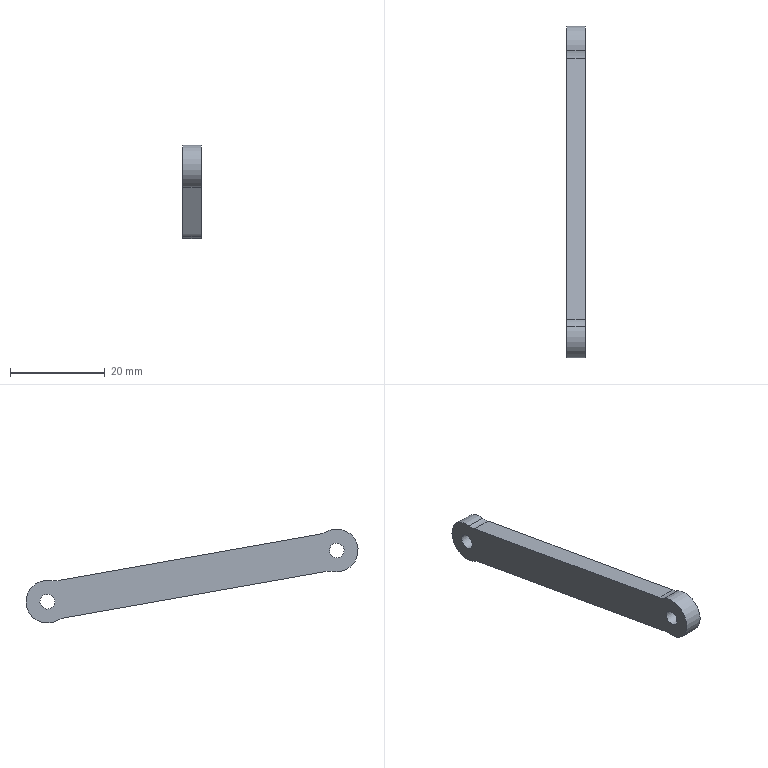Part | STEP file | Dodanie-wyci_gni_cie2_2 | 1 solid | 14 faces | box 4 x 70.047 x 19.826 mm | volume 2190 mm3 | cylinder 10 | plane 4 | commonest cylinder face diameters 9 x4 10 x4 3.1 x2
STEP:
#1=CARTESIAN_POINT('',(0.,0.,0.));
#2=DIRECTION('',(0.,0.,1.));
#3=DIRECTION('',(1.,0.,0.));
#4=AXIS2_PLACEMENT_3D('',#1,#2,#3);
#5=CARTESIAN_POINT('',(164.868,114.339,-98.824));
#6=VERTEX_POINT('',#5);
#7=CARTESIAN_POINT('',(164.868,114.609,-97.298));
#8=DIRECTION('',(1.,0.,0.));
#9=DIRECTION('',(0.,-0.1746,-0.9846));
#10=AXIS2_PLACEMENT_3D('',#7,#8,#9);
#11=CIRCLE('',#10,1.55);
#12=CARTESIAN_POINT('',(164.868,114.609,-97.298));
#13=DIRECTION('',(1.,0.,0.));
#14=DIRECTION('',(0.,-0.1746,-0.9846));
#15=AXIS2_PLACEMENT_3D('',#12,#13,#14);
#16=CYLINDRICAL_SURFACE('',#15,1.55);
#17=CARTESIAN_POINT('',(0.,0.));
#18=DIRECTION('',(1.,0.));
#19=VECTOR('',#18,1.);
#20=LINE('',#17,#19);
#21=(GEOMETRIC_REPRESENTATION_CONTEXT(2)PARAMETRIC_REPRESENTATION_CONTEXT()REPRESENTATION_CONTEXT('',''));
#22=DEFINITIONAL_REPRESENTATION('',(#20),#21);
#23=PCURVE('',#16,#22);
#24=CARTESIAN_POINT('',(164.868,145.133,-102.711));
#25=DIRECTION('',(1.,0.,0.));
#26=DIRECTION('',(0.,-0.1746,-0.9846));
#27=AXIS2_PLACEMENT_3D('',#24,#25,#26);
#28=PLANE('',#27);
#29=CARTESIAN_POINT('',(0.00000001,-31.));
#30=DIRECTION('',(1.,0.));
#31=AXIS2_PLACEMENT_2D('',#29,#30);
#32=CIRCLE('',#31,1.55);
#33=(GEOMETRIC_REPRESENTATION_CONTEXT(2)PARAMETRIC_REPRESENTATION_CONTEXT()REPRESENTATION_CONTEXT('',''));
#34=DEFINITIONAL_REPRESENTATION('',(#32),#33);
#35=PCURVE('',#28,#34);
#36=SURFACE_CURVE('',#11,(#23,#35),.PCURVE_S1.);
#37=EDGE_CURVE('',#6,#6,#36,.T.);
#38=ORIENTED_EDGE('',*,*,#37,.T.);
#39=CARTESIAN_POINT('',(168.868,114.339,-98.824));
#40=VERTEX_POINT('',#39);
#41=CARTESIAN_POINT('',(168.868,114.339,-98.824));
#42=DIRECTION('',(-1.,0.,0.));
#43=VECTOR('',#42,1.);
#44=LINE('',#41,#43);
#45=CARTESIAN_POINT('',(6.283,4.));
#46=DIRECTION('',(0.,-1.));
#47=VECTOR('',#46,1.);
#48=LINE('',#45,#47);
#49=(GEOMETRIC_REPRESENTATION_CONTEXT(2)PARAMETRIC_REPRESENTATION_CONTEXT()REPRESENTATION_CONTEXT('',''));
#50=DEFINITIONAL_REPRESENTATION('',(#48),#49);
#51=PCURVE('',#16,#50);
#52=CARTESIAN_POINT('',(0.,4.));
#53=DIRECTION('',(0.,-1.));
#54=VECTOR('',#53,1.);
#55=LINE('',#52,#54);
#56=(GEOMETRIC_REPRESENTATION_CONTEXT(2)PARAMETRIC_REPRESENTATION_CONTEXT()REPRESENTATION_CONTEXT('',''));
#57=DEFINITIONAL_REPRESENTATION('',(#55),#56);
#58=PCURVE('',#16,#57);
#59=SEAM_CURVE('',#44,(#51,#58),.PCURVE_S1.);
#60=EDGE_CURVE('',#40,#6,#59,.T.);
#61=ORIENTED_EDGE('',*,*,#60,.F.);
#62=CARTESIAN_POINT('',(168.868,114.609,-97.298));
#63=DIRECTION('',(-1.,0.,0.));
#64=DIRECTION('',(0.,-0.1746,-0.9846));
#65=AXIS2_PLACEMENT_3D('',#62,#63,#64);
#66=CIRCLE('',#65,1.55);
#67=CARTESIAN_POINT('',(6.283,4.));
#68=DIRECTION('',(-1.,0.));
#69=VECTOR('',#68,1.);
#70=LINE('',#67,#69);
#71=(GEOMETRIC_REPRESENTATION_CONTEXT(2)PARAMETRIC_REPRESENTATION_CONTEXT()REPRESENTATION_CONTEXT('',''));
#72=DEFINITIONAL_REPRESENTATION('',(#70),#71);
#73=PCURVE('',#16,#72);
#74=CARTESIAN_POINT('',(168.868,145.133,-102.711));
#75=DIRECTION('',(1.,0.,0.));
#76=DIRECTION('',(0.,-0.1746,-0.9846));
#77=AXIS2_PLACEMENT_3D('',#74,#75,#76);
#78=PLANE('',#77);
#79=CARTESIAN_POINT('',(1.55,-31.));
#80=CARTESIAN_POINT('',(1.55,-33.685));
#81=CARTESIAN_POINT('',(-0.775,-32.342));
#82=CARTESIAN_POINT('',(-3.1,-31.));
#83=CARTESIAN_POINT('',(-0.775,-29.658));
#84=CARTESIAN_POINT('',(1.55,-28.315));
#85=CARTESIAN_POINT('',(1.55,-31.));
#86=(BOUNDED_CURVE()B_SPLINE_CURVE(2,(#79,#80,#81,#82,#83,#84,#85),.UNSPECIFIED.,.T.,.F.)B_SPLINE_CURVE_WITH_KNOTS((1,2,2,2,2,1),(-2.094,0.,2.094,4.189,6.283,8.378),.UNSPECIFIED.)CURVE()GEOMETRIC_REPRESENTATION_ITEM()RATIONAL_B_SPLINE_CURVE((1.,0.5,1.,0.5,1.,0.5,1.))REPRESENTATION_ITEM(''));
#87=(GEOMETRIC_REPRESENTATION_CONTEXT(2)PARAMETRIC_REPRESENTATION_CONTEXT()REPRESENTATION_CONTEXT('',''));
#88=DEFINITIONAL_REPRESENTATION('',(#86),#87);
#89=PCURVE('',#78,#88);
#90=SURFACE_CURVE('',#66,(#73,#89),.PCURVE_S1.);
#91=EDGE_CURVE('',#40,#40,#90,.T.);
#92=ORIENTED_EDGE('',*,*,#91,.T.);
#93=ORIENTED_EDGE('',*,*,#60,.T.);
#94=EDGE_LOOP('',(#38,#61,#92,#93));
#95=FACE_BOUND('',#94,.F.);
#96=ADVANCED_FACE('',(#95),#16,.F.);
#97=CARTESIAN_POINT('',(164.868,175.386,-109.65));
#98=VERTEX_POINT('',#97);
#99=CARTESIAN_POINT('',(164.868,175.657,-108.124));
#100=DIRECTION('',(1.,0.,0.));
#101=DIRECTION('',(0.,-0.1746,-0.9846));
#102=AXIS2_PLACEMENT_3D('',#99,#100,#101);
#103=CIRCLE('',#102,1.55);
#104=CARTESIAN_POINT('',(164.868,175.657,-108.124));
#105=DIRECTION('',(1.,0.,0.));
#106=DIRECTION('',(0.,-0.1746,-0.9846));
#107=AXIS2_PLACEMENT_3D('',#104,#105,#106);
#108=CYLINDRICAL_SURFACE('',#107,1.55);
#109=CARTESIAN_POINT('',(0.,0.));
#110=DIRECTION('',(1.,0.));
#111=VECTOR('',#110,1.);
#112=LINE('',#109,#111);
#113=(GEOMETRIC_REPRESENTATION_CONTEXT(2)PARAMETRIC_REPRESENTATION_CONTEXT()REPRESENTATION_CONTEXT('',''));
#114=DEFINITIONAL_REPRESENTATION('',(#112),#113);
#115=PCURVE('',#108,#114);
#116=CARTESIAN_POINT('',(-0.00000001,31.));
#117=DIRECTION('',(1.,0.));
#118=AXIS2_PLACEMENT_2D('',#116,#117);
#119=CIRCLE('',#118,1.55);
#120=(GEOMETRIC_REPRESENTATION_CONTEXT(2)PARAMETRIC_REPRESENTATION_CONTEXT()REPRESENTATION_CONTEXT('',''));
#121=DEFINITIONAL_REPRESENTATION('',(#119),#120);
#122=PCURVE('',#28,#121);
#123=SURFACE_CURVE('',#103,(#115,#122),.PCURVE_S1.);
#124=EDGE_CURVE('',#98,#98,#123,.T.);
#125=ORIENTED_EDGE('',*,*,#124,.T.);
#126=CARTESIAN_POINT('',(168.868,175.386,-109.65));
#127=VERTEX_POINT('',#126);
#128=CARTESIAN_POINT('',(168.868,175.386,-109.65));
#129=DIRECTION('',(-1.,0.,0.));
#130=VECTOR('',#129,1.);
#131=LINE('',#128,#130);
#132=CARTESIAN_POINT('',(6.283,4.));
#133=DIRECTION('',(0.,-1.));
#134=VECTOR('',#133,1.);
#135=LINE('',#132,#134);
#136=(GEOMETRIC_REPRESENTATION_CONTEXT(2)PARAMETRIC_REPRESENTATION_CONTEXT()REPRESENTATION_CONTEXT('',''));
#137=DEFINITIONAL_REPRESENTATION('',(#135),#136);
#138=PCURVE('',#108,#137);
#139=CARTESIAN_POINT('',(0.,4.));
#140=DIRECTION('',(0.,-1.));
#141=VECTOR('',#140,1.);
#142=LINE('',#139,#141);
#143=(GEOMETRIC_REPRESENTATION_CONTEXT(2)PARAMETRIC_REPRESENTATION_CONTEXT()REPRESENTATION_CONTEXT('',''));
#144=DEFINITIONAL_REPRESENTATION('',(#142),#143);
#145=PCURVE('',#108,#144);
#146=SEAM_CURVE('',#131,(#138,#145),.PCURVE_S1.);
#147=EDGE_CURVE('',#127,#98,#146,.T.);
#148=ORIENTED_EDGE('',*,*,#147,.F.);
#149=CARTESIAN_POINT('',(168.868,175.657,-108.124));
#150=DIRECTION('',(-1.,0.,0.));
#151=DIRECTION('',(0.,-0.1746,-0.9846));
#152=AXIS2_PLACEMENT_3D('',#149,#150,#151);
#153=CIRCLE('',#152,1.55);
#154=CARTESIAN_POINT('',(6.283,4.));
#155=DIRECTION('',(-1.,0.));
#156=VECTOR('',#155,1.);
#157=LINE('',#154,#156);
#158=(GEOMETRIC_REPRESENTATION_CONTEXT(2)PARAMETRIC_REPRESENTATION_CONTEXT()REPRESENTATION_CONTEXT('',''));
#159=DEFINITIONAL_REPRESENTATION('',(#157),#158);
#160=PCURVE('',#108,#159);
#161=CARTESIAN_POINT('',(1.55,31.));
#162=CARTESIAN_POINT('',(1.55,28.315));
#163=CARTESIAN_POINT('',(-0.775,29.658));
#164=CARTESIAN_POINT('',(-3.1,31.));
#165=CARTESIAN_POINT('',(-0.775,32.342));
#166=CARTESIAN_POINT('',(1.55,33.685));
#167=CARTESIAN_POINT('',(1.55,31.));
#168=(BOUNDED_CURVE()B_SPLINE_CURVE(2,(#161,#162,#163,#164,#165,#166,#167),.UNSPECIFIED.,.T.,.F.)B_SPLINE_CURVE_WITH_KNOTS((1,2,2,2,2,1),(-2.094,0.,2.094,4.189,6.283,8.378),.UNSPECIFIED.)CURVE()GEOMETRIC_REPRESENTATION_ITEM()RATIONAL_B_SPLINE_CURVE((1.,0.5,1.,0.5,1.,0.5,1.))REPRESENTATION_ITEM(''));
#169=(GEOMETRIC_REPRESENTATION_CONTEXT(2)PARAMETRIC_REPRESENTATION_CONTEXT()REPRESENTATION_CONTEXT('',''));
#170=DEFINITIONAL_REPRESENTATION('',(#168),#169);
#171=PCURVE('',#78,#170);
#172=SURFACE_CURVE('',#153,(#160,#171),.PCURVE_S1.);
#173=EDGE_CURVE('',#127,#127,#172,.T.);
#174=ORIENTED_EDGE('',*,*,#173,.T.);
#175=ORIENTED_EDGE('',*,*,#147,.T.);
#176=EDGE_LOOP('',(#125,#148,#174,#175));
#177=FACE_BOUND('',#176,.F.);
#178=ADVANCED_FACE('',(#177),#108,.F.);
#179=CARTESIAN_POINT('',(168.868,174.871,-112.555));
#180=VERTEX_POINT('',#179);
#181=CARTESIAN_POINT('',(164.868,174.871,-112.555));
#182=VERTEX_POINT('',#181);
#183=CARTESIAN_POINT('',(168.868,174.871,-112.555));
#184=DIRECTION('',(-1.,0.,0.));
#185=VECTOR('',#184,1.);
#186=LINE('',#183,#185);
#187=CARTESIAN_POINT('',(164.868,175.657,-108.124));
#188=DIRECTION('',(1.,0.,0.));
#189=DIRECTION('',(0.,-0.1746,-0.9846));
#190=AXIS2_PLACEMENT_3D('',#187,#188,#189);
#191=CYLINDRICAL_SURFACE('',#190,4.5);
#192=CARTESIAN_POINT('',(0.,4.));
#193=DIRECTION('',(0.,-1.));
#194=VECTOR('',#193,1.);
#195=LINE('',#192,#194);
#196=(GEOMETRIC_REPRESENTATION_CONTEXT(2)PARAMETRIC_REPRESENTATION_CONTEXT()REPRESENTATION_CONTEXT('',''));
#197=DEFINITIONAL_REPRESENTATION('',(#195),#196);
#198=PCURVE('',#191,#197);
#199=CARTESIAN_POINT('',(164.868,175.657,-108.124));
#200=DIRECTION('',(1.,0.,0.));
#201=DIRECTION('',(0.,-0.1746,-0.9846));
#202=AXIS2_PLACEMENT_3D('',#199,#200,#201);
#203=CYLINDRICAL_SURFACE('',#202,4.5);
#204=CARTESIAN_POINT('',(6.283,4.));
#205=DIRECTION('',(0.,-1.));
#206=VECTOR('',#205,1.);
#207=LINE('',#204,#206);
#208=(GEOMETRIC_REPRESENTATION_CONTEXT(2)PARAMETRIC_REPRESENTATION_CONTEXT()REPRESENTATION_CONTEXT('',''));
#209=DEFINITIONAL_REPRESENTATION('',(#207),#208);
#210=PCURVE('',#203,#209);
#211=SURFACE_CURVE('',#186,(#198,#210),.PCURVE_S1.);
#212=EDGE_CURVE('',#180,#182,#211,.T.);
#213=ORIENTED_EDGE('',*,*,#212,.T.);
#214=CARTESIAN_POINT('',(164.868,174.983,-103.675));
#215=VERTEX_POINT('',#214);
#216=CARTESIAN_POINT('',(164.868,175.657,-108.124));
#217=DIRECTION('',(1.,0.,0.));
#218=DIRECTION('',(0.,-0.1746,-0.9846));
#219=AXIS2_PLACEMENT_3D('',#216,#217,#218);
#220=CIRCLE('',#219,4.5);
#221=CARTESIAN_POINT('',(0.,0.));
#222=DIRECTION('',(1.,0.));
#223=VECTOR('',#222,1.);
#224=LINE('',#221,#223);
#225=(GEOMETRIC_REPRESENTATION_CONTEXT(2)PARAMETRIC_REPRESENTATION_CONTEXT()REPRESENTATION_CONTEXT('',''));
#226=DEFINITIONAL_REPRESENTATION('',(#224),#225);
#227=PCURVE('',#191,#226);
#228=CARTESIAN_POINT('',(-0.00000001,31.));
#229=DIRECTION('',(1.,0.));
#230=AXIS2_PLACEMENT_2D('',#228,#229);
#231=CIRCLE('',#230,4.5);
#232=(GEOMETRIC_REPRESENTATION_CONTEXT(2)PARAMETRIC_REPRESENTATION_CONTEXT()REPRESENTATION_CONTEXT('',''));
#233=DEFINITIONAL_REPRESENTATION('',(#231),#232);
#234=PCURVE('',#28,#233);
#235=SURFACE_CURVE('',#220,(#227,#234),.PCURVE_S1.);
#236=EDGE_CURVE('',#182,#215,#235,.T.);
#237=ORIENTED_EDGE('',*,*,#236,.T.);
#238=CARTESIAN_POINT('',(168.868,174.983,-103.675));
#239=VERTEX_POINT('',#238);
#240=CARTESIAN_POINT('',(164.868,174.983,-103.675));
#241=DIRECTION('',(1.,0.,0.));
#242=VECTOR('',#241,1.);
#243=LINE('',#240,#242);
#244=CARTESIAN_POINT('',(3.467,0.));
#245=DIRECTION('',(0.,1.));
#246=VECTOR('',#245,1.);
#247=LINE('',#244,#246);
#248=(GEOMETRIC_REPRESENTATION_CONTEXT(2)PARAMETRIC_REPRESENTATION_CONTEXT()REPRESENTATION_CONTEXT('',''));
#249=DEFINITIONAL_REPRESENTATION('',(#247),#248);
#250=PCURVE('',#191,#249);
#251=CARTESIAN_POINT('',(164.868,174.234,-98.731));
#252=DIRECTION('',(1.,0.,0.));
#253=DIRECTION('',(0.,-0.1746,-0.9846));
#254=AXIS2_PLACEMENT_3D('',#251,#252,#253);
#255=CYLINDRICAL_SURFACE('',#254,5.);
#256=CARTESIAN_POINT('',(0.3259,0.));
#257=DIRECTION('',(0.,1.));
#258=VECTOR('',#257,1.);
#259=LINE('',#256,#258);
#260=(GEOMETRIC_REPRESENTATION_CONTEXT(2)PARAMETRIC_REPRESENTATION_CONTEXT()REPRESENTATION_CONTEXT('',''));
#261=DEFINITIONAL_REPRESENTATION('',(#259),#260);
#262=PCURVE('',#255,#261);
#263=SURFACE_CURVE('',#243,(#250,#262),.PCURVE_S1.);
#264=EDGE_CURVE('',#215,#239,#263,.T.);
#265=ORIENTED_EDGE('',*,*,#264,.T.);
#266=CARTESIAN_POINT('',(168.868,175.657,-108.124));
#267=DIRECTION('',(1.,0.,0.));
#268=DIRECTION('',(0.,-0.1746,-0.9846));
#269=AXIS2_PLACEMENT_3D('',#266,#267,#268);
#270=CIRCLE('',#269,4.5);
#271=CARTESIAN_POINT('',(0.,4.));
#272=DIRECTION('',(1.,0.));
#273=VECTOR('',#272,1.);
#274=LINE('',#271,#273);
#275=(GEOMETRIC_REPRESENTATION_CONTEXT(2)PARAMETRIC_REPRESENTATION_CONTEXT()REPRESENTATION_CONTEXT('',''));
#276=DEFINITIONAL_REPRESENTATION('',(#274),#275);
#277=PCURVE('',#191,#276);
#278=CARTESIAN_POINT('',(-0.00000001,31.));
#279=DIRECTION('',(1.,0.));
#280=AXIS2_PLACEMENT_2D('',#278,#279);
#281=CIRCLE('',#280,4.5);
#282=(GEOMETRIC_REPRESENTATION_CONTEXT(2)PARAMETRIC_REPRESENTATION_CONTEXT()REPRESENTATION_CONTEXT('',''));
#283=DEFINITIONAL_REPRESENTATION('',(#281),#282);
#284=PCURVE('',#78,#283);
#285=SURFACE_CURVE('',#270,(#277,#284),.PCURVE_S1.);
#286=EDGE_CURVE('',#180,#239,#285,.T.);
#287=ORIENTED_EDGE('',*,*,#286,.F.);
#288=EDGE_LOOP('',(#213,#237,#265,#287));
#289=FACE_BOUND('',#288,.T.);
#290=ADVANCED_FACE('',(#289),#191,.T.);
#291=CARTESIAN_POINT('',(168.868,113.823,-101.729));
#292=VERTEX_POINT('',#291);
#293=CARTESIAN_POINT('',(164.868,113.823,-101.729));
#294=VERTEX_POINT('',#293);
#295=CARTESIAN_POINT('',(168.868,113.823,-101.729));
#296=DIRECTION('',(-1.,0.,0.));
#297=VECTOR('',#296,1.);
#298=LINE('',#295,#297);
#299=CARTESIAN_POINT('',(164.868,114.609,-97.298));
#300=DIRECTION('',(1.,0.,0.));
#301=DIRECTION('',(0.,-0.1746,-0.9846));
#302=AXIS2_PLACEMENT_3D('',#299,#300,#301);
#303=CYLINDRICAL_SURFACE('',#302,4.5);
#304=CARTESIAN_POINT('',(0.,4.));
#305=DIRECTION('',(0.,-1.));
#306=VECTOR('',#305,1.);
#307=LINE('',#304,#306);
#308=(GEOMETRIC_REPRESENTATION_CONTEXT(2)PARAMETRIC_REPRESENTATION_CONTEXT()REPRESENTATION_CONTEXT('',''));
#309=DEFINITIONAL_REPRESENTATION('',(#307),#308);
#310=PCURVE('',#303,#309);
#311=CARTESIAN_POINT('',(164.868,114.609,-97.298));
#312=DIRECTION('',(1.,0.,0.));
#313=DIRECTION('',(0.,-0.1746,-0.9846));
#314=AXIS2_PLACEMENT_3D('',#311,#312,#313);
#315=CYLINDRICAL_SURFACE('',#314,4.5);
#316=CARTESIAN_POINT('',(6.283,4.));
#317=DIRECTION('',(0.,-1.));
#318=VECTOR('',#317,1.);
#319=LINE('',#316,#318);
#320=(GEOMETRIC_REPRESENTATION_CONTEXT(2)PARAMETRIC_REPRESENTATION_CONTEXT()REPRESENTATION_CONTEXT('',''));
#321=DEFINITIONAL_REPRESENTATION('',(#319),#320);
#322=PCURVE('',#315,#321);
#323=SURFACE_CURVE('',#298,(#310,#322),.PCURVE_S1.);
#324=EDGE_CURVE('',#292,#294,#323,.T.);
#325=ORIENTED_EDGE('',*,*,#324,.T.);
#326=CARTESIAN_POINT('',(164.868,115.283,-101.747));
#327=VERTEX_POINT('',#326);
#328=CARTESIAN_POINT('',(164.868,114.609,-97.298));
#329=DIRECTION('',(1.,0.,0.));
#330=DIRECTION('',(0.,-0.1746,-0.9846));
#331=AXIS2_PLACEMENT_3D('',#328,#329,#330);
#332=CIRCLE('',#331,4.5);
#333=CARTESIAN_POINT('',(0.,0.));
#334=DIRECTION('',(1.,0.));
#335=VECTOR('',#334,1.);
#336=LINE('',#333,#335);
#337=(GEOMETRIC_REPRESENTATION_CONTEXT(2)PARAMETRIC_REPRESENTATION_CONTEXT()REPRESENTATION_CONTEXT('',''));
#338=DEFINITIONAL_REPRESENTATION('',(#336),#337);
#339=PCURVE('',#303,#338);
#340=CARTESIAN_POINT('',(0.00000001,-31.));
#341=DIRECTION('',(1.,0.));
#342=AXIS2_PLACEMENT_2D('',#340,#341);
#343=CIRCLE('',#342,4.5);
#344=(GEOMETRIC_REPRESENTATION_CONTEXT(2)PARAMETRIC_REPRESENTATION_CONTEXT()REPRESENTATION_CONTEXT('',''));
#345=DEFINITIONAL_REPRESENTATION('',(#343),#344);
#346=PCURVE('',#28,#345);
#347=SURFACE_CURVE('',#332,(#339,#346),.PCURVE_S1.);
#348=EDGE_CURVE('',#294,#327,#347,.T.);
#349=ORIENTED_EDGE('',*,*,#348,.T.);
#350=CARTESIAN_POINT('',(168.868,115.283,-101.747));
#351=VERTEX_POINT('',#350);
#352=CARTESIAN_POINT('',(164.868,115.283,-101.747));
#353=DIRECTION('',(1.,0.,0.));
#354=VECTOR('',#353,1.);
#355=LINE('',#352,#354);
#356=CARTESIAN_POINT('',(0.3259,0.));
#357=DIRECTION('',(0.,1.));
#358=VECTOR('',#357,1.);
#359=LINE('',#356,#358);
#360=(GEOMETRIC_REPRESENTATION_CONTEXT(2)PARAMETRIC_REPRESENTATION_CONTEXT()REPRESENTATION_CONTEXT('',''));
#361=DEFINITIONAL_REPRESENTATION('',(#359),#360);
#362=PCURVE('',#303,#361);
#363=CARTESIAN_POINT('',(164.868,116.032,-106.691));
#364=DIRECTION('',(1.,0.,0.));
#365=DIRECTION('',(0.,-0.1746,-0.9846));
#366=AXIS2_PLACEMENT_3D('',#363,#364,#365);
#367=CYLINDRICAL_SURFACE('',#366,5.);
#368=CARTESIAN_POINT('',(3.467,0.));
#369=DIRECTION('',(0.,1.));
#370=VECTOR('',#369,1.);
#371=LINE('',#368,#370);
#372=(GEOMETRIC_REPRESENTATION_CONTEXT(2)PARAMETRIC_REPRESENTATION_CONTEXT()REPRESENTATION_CONTEXT('',''));
#373=DEFINITIONAL_REPRESENTATION('',(#371),#372);
#374=PCURVE('',#367,#373);
#375=SURFACE_CURVE('',#355,(#362,#374),.PCURVE_S1.);
#376=EDGE_CURVE('',#327,#351,#375,.T.);
#377=ORIENTED_EDGE('',*,*,#376,.T.);
#378=CARTESIAN_POINT('',(168.868,114.609,-97.298));
#379=DIRECTION('',(1.,0.,0.));
#380=DIRECTION('',(0.,-0.1746,-0.9846));
#381=AXIS2_PLACEMENT_3D('',#378,#379,#380);
#382=CIRCLE('',#381,4.5);
#383=CARTESIAN_POINT('',(0.,4.));
#384=DIRECTION('',(1.,0.));
#385=VECTOR('',#384,1.);
#386=LINE('',#383,#385);
#387=(GEOMETRIC_REPRESENTATION_CONTEXT(2)PARAMETRIC_REPRESENTATION_CONTEXT()REPRESENTATION_CONTEXT('',''));
#388=DEFINITIONAL_REPRESENTATION('',(#386),#387);
#389=PCURVE('',#303,#388);
#390=CARTESIAN_POINT('',(0.00000001,-31.));
#391=DIRECTION('',(1.,0.));
#392=AXIS2_PLACEMENT_2D('',#390,#391);
#393=CIRCLE('',#392,4.5);
#394=(GEOMETRIC_REPRESENTATION_CONTEXT(2)PARAMETRIC_REPRESENTATION_CONTEXT()REPRESENTATION_CONTEXT('',''));
#395=DEFINITIONAL_REPRESENTATION('',(#393),#394);
#396=PCURVE('',#78,#395);
#397=SURFACE_CURVE('',#382,(#389,#396),.PCURVE_S1.);
#398=EDGE_CURVE('',#292,#351,#397,.T.);
#399=ORIENTED_EDGE('',*,*,#398,.F.);
#400=EDGE_LOOP('',(#325,#349,#377,#399));
#401=FACE_BOUND('',#400,.T.);
#402=ADVANCED_FACE('',(#401),#303,.T.);
#403=ORIENTED_EDGE('',*,*,#91,.T.);
#404=EDGE_LOOP('',(#403));
#405=FACE_BOUND('',#404,.T.);
#406=ORIENTED_EDGE('',*,*,#173,.T.);
#407=EDGE_LOOP('',(#406));
#408=FACE_BOUND('',#407,.T.);
#409=CARTESIAN_POINT('',(168.868,173.361,-103.655));
#410=VERTEX_POINT('',#409);
#411=CARTESIAN_POINT('',(168.868,118.302,-93.89));
#412=VERTEX_POINT('',#411);
#413=CARTESIAN_POINT('',(168.868,173.361,-103.655));
#414=DIRECTION('',(0.,-0.9846,0.1746));
#415=VECTOR('',#414,1.);
#416=LINE('',#413,#415);
#417=CARTESIAN_POINT('',(-4.,27.959));
#418=DIRECTION('',(0.,-1.));
#419=VECTOR('',#418,1.);
#420=LINE('',#417,#419);
#421=(GEOMETRIC_REPRESENTATION_CONTEXT(2)PARAMETRIC_REPRESENTATION_CONTEXT()REPRESENTATION_CONTEXT('',''));
#422=DEFINITIONAL_REPRESENTATION('',(#420),#421);
#423=PCURVE('',#78,#422);
#424=CARTESIAN_POINT('',(166.868,145.831,-98.773));
#425=DIRECTION('',(0.,0.1746,0.9846));
#426=DIRECTION('',(1.,0.,0.));
#427=AXIS2_PLACEMENT_3D('',#424,#425,#426);
#428=PLANE('',#427);
#429=CARTESIAN_POINT('',(2.,27.959));
#430=DIRECTION('',(0.,-1.));
#431=VECTOR('',#430,1.);
#432=LINE('',#429,#431);
#433=(GEOMETRIC_REPRESENTATION_CONTEXT(2)PARAMETRIC_REPRESENTATION_CONTEXT()REPRESENTATION_CONTEXT('',''));
#434=DEFINITIONAL_REPRESENTATION('',(#432),#433);
#435=PCURVE('',#428,#434);
#436=SURFACE_CURVE('',#416,(#423,#435),.PCURVE_S1.);
#437=EDGE_CURVE('',#410,#412,#436,.T.);
#438=ORIENTED_EDGE('',*,*,#437,.T.);
#439=CARTESIAN_POINT('',(168.868,116.772,-93.352));
#440=VERTEX_POINT('',#439);
#441=CARTESIAN_POINT('',(168.868,119.175,-88.967));
#442=DIRECTION('',(-1.,0.,0.));
#443=DIRECTION('',(0.,-0.1746,-0.9846));
#444=AXIS2_PLACEMENT_3D('',#441,#442,#443);
#445=CIRCLE('',#444,5.);
#446=CARTESIAN_POINT('',(-4.,-27.959));
#447=CARTESIAN_POINT('',(-4.,-36.619));
#448=CARTESIAN_POINT('',(-11.5,-32.289));
#449=CARTESIAN_POINT('',(-19.,-27.959));
#450=CARTESIAN_POINT('',(-11.5,-23.628));
#451=CARTESIAN_POINT('',(-4.,-19.298));
#452=CARTESIAN_POINT('',(-4.,-27.959));
#453=(BOUNDED_CURVE()B_SPLINE_CURVE(2,(#446,#447,#448,#449,#450,#451,#452),.UNSPECIFIED.,.T.,.F.)B_SPLINE_CURVE_WITH_KNOTS((1,2,2,2,2,1),(-2.094,0.,2.094,4.189,6.283,8.378),.UNSPECIFIED.)CURVE()GEOMETRIC_REPRESENTATION_ITEM()RATIONAL_B_SPLINE_CURVE((1.,0.5,1.,0.5,1.,0.5,1.))REPRESENTATION_ITEM(''));
#454=(GEOMETRIC_REPRESENTATION_CONTEXT(2)PARAMETRIC_REPRESENTATION_CONTEXT()REPRESENTATION_CONTEXT('',''));
#455=DEFINITIONAL_REPRESENTATION('',(#453),#454);
#456=PCURVE('',#78,#455);
#457=CARTESIAN_POINT('',(164.868,119.175,-88.967));
#458=DIRECTION('',(1.,0.,0.));
#459=DIRECTION('',(0.,-0.1746,-0.9846));
#460=AXIS2_PLACEMENT_3D('',#457,#458,#459);
#461=CYLINDRICAL_SURFACE('',#460,5.);
#462=CARTESIAN_POINT('',(6.283,4.));
#463=DIRECTION('',(-1.,0.));
#464=VECTOR('',#463,1.);
#465=LINE('',#462,#464);
#466=(GEOMETRIC_REPRESENTATION_CONTEXT(2)PARAMETRIC_REPRESENTATION_CONTEXT()REPRESENTATION_CONTEXT('',''));
#467=DEFINITIONAL_REPRESENTATION('',(#465),#466);
#468=PCURVE('',#461,#467);
#469=SURFACE_CURVE('',#445,(#456,#468),.PCURVE_S1.);
#470=EDGE_CURVE('',#412,#440,#469,.T.);
#471=ORIENTED_EDGE('',*,*,#470,.T.);
#472=CARTESIAN_POINT('',(168.868,114.609,-97.298));
#473=DIRECTION('',(1.,0.,0.));
#474=DIRECTION('',(0.,-0.1746,-0.9846));
#475=AXIS2_PLACEMENT_3D('',#472,#473,#474);
#476=CIRCLE('',#475,4.5);
#477=CARTESIAN_POINT('',(0.00000001,-31.));
#478=DIRECTION('',(1.,0.));
#479=AXIS2_PLACEMENT_2D('',#477,#478);
#480=CIRCLE('',#479,4.5);
#481=(GEOMETRIC_REPRESENTATION_CONTEXT(2)PARAMETRIC_REPRESENTATION_CONTEXT()REPRESENTATION_CONTEXT('',''));
#482=DEFINITIONAL_REPRESENTATION('',(#480),#481);
#483=PCURVE('',#78,#482);
#484=CARTESIAN_POINT('',(0.,4.));
#485=DIRECTION('',(1.,0.));
#486=VECTOR('',#485,1.);
#487=LINE('',#484,#486);
#488=(GEOMETRIC_REPRESENTATION_CONTEXT(2)PARAMETRIC_REPRESENTATION_CONTEXT()REPRESENTATION_CONTEXT('',''));
#489=DEFINITIONAL_REPRESENTATION('',(#487),#488);
#490=PCURVE('',#315,#489);
#491=SURFACE_CURVE('',#476,(#483,#490),.PCURVE_S1.);
#492=EDGE_CURVE('',#440,#292,#491,.T.);
#493=ORIENTED_EDGE('',*,*,#492,.T.);
#494=ORIENTED_EDGE('',*,*,#398,.T.);
#495=CARTESIAN_POINT('',(168.868,116.905,-101.768));
#496=VERTEX_POINT('',#495);
#497=CARTESIAN_POINT('',(168.868,116.032,-106.691));
#498=DIRECTION('',(-1.,0.,0.));
#499=DIRECTION('',(0.,-0.1746,-0.9846));
#500=AXIS2_PLACEMENT_3D('',#497,#498,#499);
#501=CIRCLE('',#500,5.);
#502=CARTESIAN_POINT('',(14.,-27.959));
#503=CARTESIAN_POINT('',(14.,-36.619));
#504=CARTESIAN_POINT('',(6.5,-32.289));
#505=CARTESIAN_POINT('',(-1.,-27.959));
#506=CARTESIAN_POINT('',(6.5,-23.628));
#507=CARTESIAN_POINT('',(14.,-19.298));
#508=CARTESIAN_POINT('',(14.,-27.959));
#509=(BOUNDED_CURVE()B_SPLINE_CURVE(2,(#502,#503,#504,#505,#506,#507,#508),.UNSPECIFIED.,.T.,.F.)B_SPLINE_CURVE_WITH_KNOTS((1,2,2,2,2,1),(-2.094,0.,2.094,4.189,6.283,8.378),.UNSPECIFIED.)CURVE()GEOMETRIC_REPRESENTATION_ITEM()RATIONAL_B_SPLINE_CURVE((1.,0.5,1.,0.5,1.,0.5,1.))REPRESENTATION_ITEM(''));
#510=(GEOMETRIC_REPRESENTATION_CONTEXT(2)PARAMETRIC_REPRESENTATION_CONTEXT()REPRESENTATION_CONTEXT('',''));
#511=DEFINITIONAL_REPRESENTATION('',(#509),#510);
#512=PCURVE('',#78,#511);
#513=CARTESIAN_POINT('',(6.283,4.));
#514=DIRECTION('',(-1.,0.));
#515=VECTOR('',#514,1.);
#516=LINE('',#513,#515);
#517=(GEOMETRIC_REPRESENTATION_CONTEXT(2)PARAMETRIC_REPRESENTATION_CONTEXT()REPRESENTATION_CONTEXT('',''));
#518=DEFINITIONAL_REPRESENTATION('',(#516),#517);
#519=PCURVE('',#367,#518);
#520=SURFACE_CURVE('',#501,(#512,#519),.PCURVE_S1.);
#521=EDGE_CURVE('',#351,#496,#520,.T.);
#522=ORIENTED_EDGE('',*,*,#521,.T.);
#523=CARTESIAN_POINT('',(168.868,171.964,-111.532));
#524=VERTEX_POINT('',#523);
#525=CARTESIAN_POINT('',(168.868,116.905,-101.768));
#526=DIRECTION('',(0.,0.9846,-0.1746));
#527=VECTOR('',#526,1.);
#528=LINE('',#525,#527);
#529=CARTESIAN_POINT('',(4.,-27.959));
#530=DIRECTION('',(0.,1.));
#531=VECTOR('',#530,1.);
#532=LINE('',#529,#531);
#533=(GEOMETRIC_REPRESENTATION_CONTEXT(2)PARAMETRIC_REPRESENTATION_CONTEXT()REPRESENTATION_CONTEXT('',''));
#534=DEFINITIONAL_REPRESENTATION('',(#532),#533);
#535=PCURVE('',#78,#534);
#536=CARTESIAN_POINT('',(166.868,144.435,-106.65));
#537=DIRECTION('',(0.,-0.1746,-0.9846));
#538=DIRECTION('',(-1.,0.,0.));
#539=AXIS2_PLACEMENT_3D('',#536,#537,#538);
#540=PLANE('',#539);
#541=CARTESIAN_POINT('',(-2.,-27.959));
#542=DIRECTION('',(0.,1.));
#543=VECTOR('',#542,1.);
#544=LINE('',#541,#543);
#545=(GEOMETRIC_REPRESENTATION_CONTEXT(2)PARAMETRIC_REPRESENTATION_CONTEXT()REPRESENTATION_CONTEXT('',''));
#546=DEFINITIONAL_REPRESENTATION('',(#544),#545);
#547=PCURVE('',#540,#546);
#548=SURFACE_CURVE('',#528,(#535,#547),.PCURVE_S1.);
#549=EDGE_CURVE('',#496,#524,#548,.T.);
#550=ORIENTED_EDGE('',*,*,#549,.T.);
#551=CARTESIAN_POINT('',(168.868,173.494,-112.07));
#552=VERTEX_POINT('',#551);
#553=CARTESIAN_POINT('',(168.868,171.091,-116.455));
#554=DIRECTION('',(-1.,0.,0.));
#555=DIRECTION('',(0.,-0.1746,-0.9846));
#556=AXIS2_PLACEMENT_3D('',#553,#554,#555);
#557=CIRCLE('',#556,5.);
#558=CARTESIAN_POINT('',(14.,27.959));
#559=CARTESIAN_POINT('',(14.,19.298));
#560=CARTESIAN_POINT('',(6.5,23.628));
#561=CARTESIAN_POINT('',(-1.,27.959));
#562=CARTESIAN_POINT('',(6.5,32.289));
#563=CARTESIAN_POINT('',(14.,36.619));
#564=CARTESIAN_POINT('',(14.,27.959));
#565=(BOUNDED_CURVE()B_SPLINE_CURVE(2,(#558,#559,#560,#561,#562,#563,#564),.UNSPECIFIED.,.T.,.F.)B_SPLINE_CURVE_WITH_KNOTS((1,2,2,2,2,1),(-2.094,0.,2.094,4.189,6.283,8.378),.UNSPECIFIED.)CURVE()GEOMETRIC_REPRESENTATION_ITEM()RATIONAL_B_SPLINE_CURVE((1.,0.5,1.,0.5,1.,0.5,1.))REPRESENTATION_ITEM(''));
#566=(GEOMETRIC_REPRESENTATION_CONTEXT(2)PARAMETRIC_REPRESENTATION_CONTEXT()REPRESENTATION_CONTEXT('',''));
#567=DEFINITIONAL_REPRESENTATION('',(#565),#566);
#568=PCURVE('',#78,#567);
#569=CARTESIAN_POINT('',(164.868,171.091,-116.455));
#570=DIRECTION('',(1.,0.,0.));
#571=DIRECTION('',(0.,-0.1746,-0.9846));
#572=AXIS2_PLACEMENT_3D('',#569,#570,#571);
#573=CYLINDRICAL_SURFACE('',#572,5.);
#574=CARTESIAN_POINT('',(6.283,4.));
#575=DIRECTION('',(-1.,0.));
#576=VECTOR('',#575,1.);
#577=LINE('',#574,#576);
#578=(GEOMETRIC_REPRESENTATION_CONTEXT(2)PARAMETRIC_REPRESENTATION_CONTEXT()REPRESENTATION_CONTEXT('',''));
#579=DEFINITIONAL_REPRESENTATION('',(#577),#578);
#580=PCURVE('',#573,#579);
#581=SURFACE_CURVE('',#557,(#568,#580),.PCURVE_S1.);
#582=EDGE_CURVE('',#524,#552,#581,.T.);
#583=ORIENTED_EDGE('',*,*,#582,.T.);
#584=CARTESIAN_POINT('',(168.868,175.657,-108.124));
#585=DIRECTION('',(1.,0.,0.));
#586=DIRECTION('',(0.,-0.1746,-0.9846));
#587=AXIS2_PLACEMENT_3D('',#584,#585,#586);
#588=CIRCLE('',#587,4.5);
#589=CARTESIAN_POINT('',(-0.00000001,31.));
#590=DIRECTION('',(1.,0.));
#591=AXIS2_PLACEMENT_2D('',#589,#590);
#592=CIRCLE('',#591,4.5);
#593=(GEOMETRIC_REPRESENTATION_CONTEXT(2)PARAMETRIC_REPRESENTATION_CONTEXT()REPRESENTATION_CONTEXT('',''));
#594=DEFINITIONAL_REPRESENTATION('',(#592),#593);
#595=PCURVE('',#78,#594);
#596=CARTESIAN_POINT('',(0.,4.));
#597=DIRECTION('',(1.,0.));
#598=VECTOR('',#597,1.);
#599=LINE('',#596,#598);
#600=(GEOMETRIC_REPRESENTATION_CONTEXT(2)PARAMETRIC_REPRESENTATION_CONTEXT()REPRESENTATION_CONTEXT('',''));
#601=DEFINITIONAL_REPRESENTATION('',(#599),#600);
#602=PCURVE('',#203,#601);
#603=SURFACE_CURVE('',#588,(#595,#602),.PCURVE_S1.);
#604=EDGE_CURVE('',#552,#180,#603,.T.);
#605=ORIENTED_EDGE('',*,*,#604,.T.);
#606=ORIENTED_EDGE('',*,*,#286,.T.);
#607=CARTESIAN_POINT('',(168.868,174.234,-98.731));
#608=DIRECTION('',(-1.,0.,0.));
#609=DIRECTION('',(0.,-0.1746,-0.9846));
#610=AXIS2_PLACEMENT_3D('',#607,#608,#609);
#611=CIRCLE('',#610,5.);
#612=CARTESIAN_POINT('',(-4.,27.959));
#613=CARTESIAN_POINT('',(-4.,19.298));
#614=CARTESIAN_POINT('',(-11.5,23.628));
#615=CARTESIAN_POINT('',(-19.,27.959));
#616=CARTESIAN_POINT('',(-11.5,32.289));
#617=CARTESIAN_POINT('',(-4.,36.619));
#618=CARTESIAN_POINT('',(-4.,27.959));
#619=(BOUNDED_CURVE()B_SPLINE_CURVE(2,(#612,#613,#614,#615,#616,#617,#618),.UNSPECIFIED.,.T.,.F.)B_SPLINE_CURVE_WITH_KNOTS((1,2,2,2,2,1),(-2.094,0.,2.094,4.189,6.283,8.378),.UNSPECIFIED.)CURVE()GEOMETRIC_REPRESENTATION_ITEM()RATIONAL_B_SPLINE_CURVE((1.,0.5,1.,0.5,1.,0.5,1.))REPRESENTATION_ITEM(''));
#620=(GEOMETRIC_REPRESENTATION_CONTEXT(2)PARAMETRIC_REPRESENTATION_CONTEXT()REPRESENTATION_CONTEXT('',''));
#621=DEFINITIONAL_REPRESENTATION('',(#619),#620);
#622=PCURVE('',#78,#621);
#623=CARTESIAN_POINT('',(6.283,4.));
#624=DIRECTION('',(-1.,0.));
#625=VECTOR('',#624,1.);
#626=LINE('',#623,#625);
#627=(GEOMETRIC_REPRESENTATION_CONTEXT(2)PARAMETRIC_REPRESENTATION_CONTEXT()REPRESENTATION_CONTEXT('',''));
#628=DEFINITIONAL_REPRESENTATION('',(#626),#627);
#629=PCURVE('',#255,#628);
#630=SURFACE_CURVE('',#611,(#622,#629),.PCURVE_S1.);
#631=EDGE_CURVE('',#239,#410,#630,.T.);
#632=ORIENTED_EDGE('',*,*,#631,.T.);
#633=EDGE_LOOP('',(#438,#471,#493,#494,#522,#550,#583,#605,#606,#632));
#634=FACE_BOUND('',#633,.T.);
#635=ADVANCED_FACE('',(#405,#408,#634),#78,.T.);
#636=ORIENTED_EDGE('',*,*,#437,.F.);
#637=CARTESIAN_POINT('',(164.868,173.361,-103.655));
#638=VERTEX_POINT('',#637);
#639=CARTESIAN_POINT('',(168.868,173.361,-103.655));
#640=DIRECTION('',(-1.,0.,0.));
#641=VECTOR('',#640,1.);
#642=LINE('',#639,#641);
#643=CARTESIAN_POINT('',(2.,27.959));
#644=DIRECTION('',(-1.,0.));
#645=VECTOR('',#644,1.);
#646=LINE('',#643,#645);
#647=(GEOMETRIC_REPRESENTATION_CONTEXT(2)PARAMETRIC_REPRESENTATION_CONTEXT()REPRESENTATION_CONTEXT('',''));
#648=DEFINITIONAL_REPRESENTATION('',(#646),#647);
#649=PCURVE('',#428,#648);
#650=CARTESIAN_POINT('',(0.,4.));
#651=DIRECTION('',(0.,-1.));
#652=VECTOR('',#651,1.);
#653=LINE('',#650,#652);
#654=(GEOMETRIC_REPRESENTATION_CONTEXT(2)PARAMETRIC_REPRESENTATION_CONTEXT()REPRESENTATION_CONTEXT('',''));
#655=DEFINITIONAL_REPRESENTATION('',(#653),#654);
#656=PCURVE('',#255,#655);
#657=SURFACE_CURVE('',#642,(#649,#656),.PCURVE_S1.);
#658=EDGE_CURVE('',#410,#638,#657,.T.);
#659=ORIENTED_EDGE('',*,*,#658,.T.);
#660=CARTESIAN_POINT('',(164.868,118.302,-93.89));
#661=VERTEX_POINT('',#660);
#662=CARTESIAN_POINT('',(164.868,173.361,-103.655));
#663=DIRECTION('',(0.,-0.9846,0.1746));
#664=VECTOR('',#663,1.);
#665=LINE('',#662,#664);
#666=CARTESIAN_POINT('',(-2.,27.959));
#667=DIRECTION('',(0.,-1.));
#668=VECTOR('',#667,1.);
#669=LINE('',#666,#668);
#670=(GEOMETRIC_REPRESENTATION_CONTEXT(2)PARAMETRIC_REPRESENTATION_CONTEXT()REPRESENTATION_CONTEXT('',''));
#671=DEFINITIONAL_REPRESENTATION('',(#669),#670);
#672=PCURVE('',#428,#671);
#673=CARTESIAN_POINT('',(-4.,27.959));
#674=DIRECTION('',(0.,-1.));
#675=VECTOR('',#674,1.);
#676=LINE('',#673,#675);
#677=(GEOMETRIC_REPRESENTATION_CONTEXT(2)PARAMETRIC_REPRESENTATION_CONTEXT()REPRESENTATION_CONTEXT('',''));
#678=DEFINITIONAL_REPRESENTATION('',(#676),#677);
#679=PCURVE('',#28,#678);
#680=SURFACE_CURVE('',#665,(#672,#679),.PCURVE_S1.);
#681=EDGE_CURVE('',#638,#661,#680,.T.);
#682=ORIENTED_EDGE('',*,*,#681,.T.);
#683=CARTESIAN_POINT('',(164.868,118.302,-93.89));
#684=DIRECTION('',(1.,0.,0.));
#685=VECTOR('',#684,1.);
#686=LINE('',#683,#685);
#687=CARTESIAN_POINT('',(-2.,-27.959));
#688=DIRECTION('',(1.,0.));
#689=VECTOR('',#688,1.);
#690=LINE('',#687,#689);
#691=(GEOMETRIC_REPRESENTATION_CONTEXT(2)PARAMETRIC_REPRESENTATION_CONTEXT()REPRESENTATION_CONTEXT('',''));
#692=DEFINITIONAL_REPRESENTATION('',(#690),#691);
#693=PCURVE('',#428,#692);
#694=CARTESIAN_POINT('',(6.283,0.));
#695=DIRECTION('',(0.,1.));
#696=VECTOR('',#695,1.);
#697=LINE('',#694,#696);
#698=(GEOMETRIC_REPRESENTATION_CONTEXT(2)PARAMETRIC_REPRESENTATION_CONTEXT()REPRESENTATION_CONTEXT('',''));
#699=DEFINITIONAL_REPRESENTATION('',(#697),#698);
#700=PCURVE('',#461,#699);
#701=SURFACE_CURVE('',#686,(#693,#700),.PCURVE_S1.);
#702=EDGE_CURVE('',#661,#412,#701,.T.);
#703=ORIENTED_EDGE('',*,*,#702,.T.);
#704=EDGE_LOOP('',(#636,#659,#682,#703));
#705=FACE_BOUND('',#704,.T.);
#706=ADVANCED_FACE('',(#705),#428,.T.);
#707=CARTESIAN_POINT('',(164.868,116.905,-101.768));
#708=VERTEX_POINT('',#707);
#709=CARTESIAN_POINT('',(164.868,171.964,-111.532));
#710=VERTEX_POINT('',#709);
#711=CARTESIAN_POINT('',(164.868,116.905,-101.768));
#712=DIRECTION('',(0.,0.9846,-0.1746));
#713=VECTOR('',#712,1.);
#714=LINE('',#711,#713);
#715=CARTESIAN_POINT('',(2.,-27.959));
#716=DIRECTION('',(0.,1.));
#717=VECTOR('',#716,1.);
#718=LINE('',#715,#717);
#719=(GEOMETRIC_REPRESENTATION_CONTEXT(2)PARAMETRIC_REPRESENTATION_CONTEXT()REPRESENTATION_CONTEXT('',''));
#720=DEFINITIONAL_REPRESENTATION('',(#718),#719);
#721=PCURVE('',#540,#720);
#722=CARTESIAN_POINT('',(4.,-27.959));
#723=DIRECTION('',(0.,1.));
#724=VECTOR('',#723,1.);
#725=LINE('',#722,#724);
#726=(GEOMETRIC_REPRESENTATION_CONTEXT(2)PARAMETRIC_REPRESENTATION_CONTEXT()REPRESENTATION_CONTEXT('',''));
#727=DEFINITIONAL_REPRESENTATION('',(#725),#726);
#728=PCURVE('',#28,#727);
#729=SURFACE_CURVE('',#714,(#721,#728),.PCURVE_S1.);
#730=EDGE_CURVE('',#708,#710,#729,.T.);
#731=ORIENTED_EDGE('',*,*,#730,.T.);
#732=CARTESIAN_POINT('',(164.868,171.964,-111.532));
#733=DIRECTION('',(1.,0.,0.));
#734=VECTOR('',#733,1.);
#735=LINE('',#732,#734);
#736=CARTESIAN_POINT('',(2.,27.959));
#737=DIRECTION('',(-1.,0.));
#738=VECTOR('',#737,1.);
#739=LINE('',#736,#738);
#740=(GEOMETRIC_REPRESENTATION_CONTEXT(2)PARAMETRIC_REPRESENTATION_CONTEXT()REPRESENTATION_CONTEXT('',''));
#741=DEFINITIONAL_REPRESENTATION('',(#739),#740);
#742=PCURVE('',#540,#741);
#743=CARTESIAN_POINT('',(3.142,0.));
#744=DIRECTION('',(0.,1.));
#745=VECTOR('',#744,1.);
#746=LINE('',#743,#745);
#747=(GEOMETRIC_REPRESENTATION_CONTEXT(2)PARAMETRIC_REPRESENTATION_CONTEXT()REPRESENTATION_CONTEXT('',''));
#748=DEFINITIONAL_REPRESENTATION('',(#746),#747);
#749=PCURVE('',#573,#748);
#750=SURFACE_CURVE('',#735,(#742,#749),.PCURVE_S1.);
#751=EDGE_CURVE('',#710,#524,#750,.T.);
#752=ORIENTED_EDGE('',*,*,#751,.T.);
#753=ORIENTED_EDGE('',*,*,#549,.F.);
#754=CARTESIAN_POINT('',(168.868,116.905,-101.768));
#755=DIRECTION('',(-1.,0.,0.));
#756=VECTOR('',#755,1.);
#757=LINE('',#754,#756);
#758=CARTESIAN_POINT('',(-2.,-27.959));
#759=DIRECTION('',(1.,0.));
#760=VECTOR('',#759,1.);
#761=LINE('',#758,#760);
#762=(GEOMETRIC_REPRESENTATION_CONTEXT(2)PARAMETRIC_REPRESENTATION_CONTEXT()REPRESENTATION_CONTEXT('',''));
#763=DEFINITIONAL_REPRESENTATION('',(#761),#762);
#764=PCURVE('',#540,#763);
#765=CARTESIAN_POINT('',(3.142,4.));
#766=DIRECTION('',(0.,-1.));
#767=VECTOR('',#766,1.);
#768=LINE('',#765,#767);
#769=(GEOMETRIC_REPRESENTATION_CONTEXT(2)PARAMETRIC_REPRESENTATION_CONTEXT()REPRESENTATION_CONTEXT('',''));
#770=DEFINITIONAL_REPRESENTATION('',(#768),#769);
#771=PCURVE('',#367,#770);
#772=SURFACE_CURVE('',#757,(#764,#771),.PCURVE_S1.);
#773=EDGE_CURVE('',#496,#708,#772,.T.);
#774=ORIENTED_EDGE('',*,*,#773,.T.);
#775=EDGE_LOOP('',(#731,#752,#753,#774));
#776=FACE_BOUND('',#775,.T.);
#777=ADVANCED_FACE('',(#776),#540,.T.);
#778=ORIENTED_EDGE('',*,*,#37,.T.);
#779=EDGE_LOOP('',(#778));
#780=FACE_BOUND('',#779,.T.);
#781=ORIENTED_EDGE('',*,*,#124,.T.);
#782=EDGE_LOOP('',(#781));
#783=FACE_BOUND('',#782,.T.);
#784=CARTESIAN_POINT('',(164.868,116.772,-93.352));
#785=VERTEX_POINT('',#784);
#786=CARTESIAN_POINT('',(164.868,119.175,-88.967));
#787=DIRECTION('',(-1.,0.,0.));
#788=DIRECTION('',(0.,-0.1746,-0.9846));
#789=AXIS2_PLACEMENT_3D('',#786,#787,#788);
#790=CIRCLE('',#789,5.);
#791=CARTESIAN_POINT('',(-4.,-27.959));
#792=CARTESIAN_POINT('',(-4.,-36.619));
#793=CARTESIAN_POINT('',(-11.5,-32.289));
#794=CARTESIAN_POINT('',(-19.,-27.959));
#795=CARTESIAN_POINT('',(-11.5,-23.628));
#796=CARTESIAN_POINT('',(-4.,-19.298));
#797=CARTESIAN_POINT('',(-4.,-27.959));
#798=(BOUNDED_CURVE()B_SPLINE_CURVE(2,(#791,#792,#793,#794,#795,#796,#797),.UNSPECIFIED.,.T.,.F.)B_SPLINE_CURVE_WITH_KNOTS((1,2,2,2,2,1),(-2.094,0.,2.094,4.189,6.283,8.378),.UNSPECIFIED.)CURVE()GEOMETRIC_REPRESENTATION_ITEM()RATIONAL_B_SPLINE_CURVE((1.,0.5,1.,0.5,1.,0.5,1.))REPRESENTATION_ITEM(''));
#799=(GEOMETRIC_REPRESENTATION_CONTEXT(2)PARAMETRIC_REPRESENTATION_CONTEXT()REPRESENTATION_CONTEXT('',''));
#800=DEFINITIONAL_REPRESENTATION('',(#798),#799);
#801=PCURVE('',#28,#800);
#802=CARTESIAN_POINT('',(6.283,0.));
#803=DIRECTION('',(-1.,0.));
#804=VECTOR('',#803,1.);
#805=LINE('',#802,#804);
#806=(GEOMETRIC_REPRESENTATION_CONTEXT(2)PARAMETRIC_REPRESENTATION_CONTEXT()REPRESENTATION_CONTEXT('',''));
#807=DEFINITIONAL_REPRESENTATION('',(#805),#806);
#808=PCURVE('',#461,#807);
#809=SURFACE_CURVE('',#790,(#801,#808),.PCURVE_S1.);
#810=EDGE_CURVE('',#661,#785,#809,.T.);
#811=ORIENTED_EDGE('',*,*,#810,.F.);
#812=ORIENTED_EDGE('',*,*,#681,.F.);
#813=CARTESIAN_POINT('',(164.868,174.234,-98.731));
#814=DIRECTION('',(-1.,0.,0.));
#815=DIRECTION('',(0.,-0.1746,-0.9846));
#816=AXIS2_PLACEMENT_3D('',#813,#814,#815);
#817=CIRCLE('',#816,5.);
#818=CARTESIAN_POINT('',(-4.,27.959));
#819=CARTESIAN_POINT('',(-4.,19.298));
#820=CARTESIAN_POINT('',(-11.5,23.628));
#821=CARTESIAN_POINT('',(-19.,27.959));
#822=CARTESIAN_POINT('',(-11.5,32.289));
#823=CARTESIAN_POINT('',(-4.,36.619));
#824=CARTESIAN_POINT('',(-4.,27.959));
#825=(BOUNDED_CURVE()B_SPLINE_CURVE(2,(#818,#819,#820,#821,#822,#823,#824),.UNSPECIFIED.,.T.,.F.)B_SPLINE_CURVE_WITH_KNOTS((1,2,2,2,2,1),(-2.094,0.,2.094,4.189,6.283,8.378),.UNSPECIFIED.)CURVE()GEOMETRIC_REPRESENTATION_ITEM()RATIONAL_B_SPLINE_CURVE((1.,0.5,1.,0.5,1.,0.5,1.))REPRESENTATION_ITEM(''));
#826=(GEOMETRIC_REPRESENTATION_CONTEXT(2)PARAMETRIC_REPRESENTATION_CONTEXT()REPRESENTATION_CONTEXT('',''));
#827=DEFINITIONAL_REPRESENTATION('',(#825),#826);
#828=PCURVE('',#28,#827);
#829=CARTESIAN_POINT('',(6.283,0.));
#830=DIRECTION('',(-1.,0.));
#831=VECTOR('',#830,1.);
#832=LINE('',#829,#831);
#833=(GEOMETRIC_REPRESENTATION_CONTEXT(2)PARAMETRIC_REPRESENTATION_CONTEXT()REPRESENTATION_CONTEXT('',''));
#834=DEFINITIONAL_REPRESENTATION('',(#832),#833);
#835=PCURVE('',#255,#834);
#836=SURFACE_CURVE('',#817,(#828,#835),.PCURVE_S1.);
#837=EDGE_CURVE('',#215,#638,#836,.T.);
#838=ORIENTED_EDGE('',*,*,#837,.F.);
#839=ORIENTED_EDGE('',*,*,#236,.F.);
#840=CARTESIAN_POINT('',(164.868,173.494,-112.07));
#841=VERTEX_POINT('',#840);
#842=CARTESIAN_POINT('',(164.868,175.657,-108.124));
#843=DIRECTION('',(1.,0.,0.));
#844=DIRECTION('',(0.,-0.1746,-0.9846));
#845=AXIS2_PLACEMENT_3D('',#842,#843,#844);
#846=CIRCLE('',#845,4.5);
#847=CARTESIAN_POINT('',(-0.00000001,31.));
#848=DIRECTION('',(1.,0.));
#849=AXIS2_PLACEMENT_2D('',#847,#848);
#850=CIRCLE('',#849,4.5);
#851=(GEOMETRIC_REPRESENTATION_CONTEXT(2)PARAMETRIC_REPRESENTATION_CONTEXT()REPRESENTATION_CONTEXT('',''));
#852=DEFINITIONAL_REPRESENTATION('',(#850),#851);
#853=PCURVE('',#28,#852);
#854=CARTESIAN_POINT('',(0.,0.));
#855=DIRECTION('',(1.,0.));
#856=VECTOR('',#855,1.);
#857=LINE('',#854,#856);
#858=(GEOMETRIC_REPRESENTATION_CONTEXT(2)PARAMETRIC_REPRESENTATION_CONTEXT()REPRESENTATION_CONTEXT('',''));
#859=DEFINITIONAL_REPRESENTATION('',(#857),#858);
#860=PCURVE('',#203,#859);
#861=SURFACE_CURVE('',#846,(#853,#860),.PCURVE_S1.);
#862=EDGE_CURVE('',#841,#182,#861,.T.);
#863=ORIENTED_EDGE('',*,*,#862,.F.);
#864=CARTESIAN_POINT('',(164.868,171.091,-116.455));
#865=DIRECTION('',(-1.,0.,0.));
#866=DIRECTION('',(0.,-0.1746,-0.9846));
#867=AXIS2_PLACEMENT_3D('',#864,#865,#866);
#868=CIRCLE('',#867,5.);
#869=CARTESIAN_POINT('',(14.,27.959));
#870=CARTESIAN_POINT('',(14.,19.298));
#871=CARTESIAN_POINT('',(6.5,23.628));
#872=CARTESIAN_POINT('',(-1.,27.959));
#873=CARTESIAN_POINT('',(6.5,32.289));
#874=CARTESIAN_POINT('',(14.,36.619));
#875=CARTESIAN_POINT('',(14.,27.959));
#876=(BOUNDED_CURVE()B_SPLINE_CURVE(2,(#869,#870,#871,#872,#873,#874,#875),.UNSPECIFIED.,.T.,.F.)B_SPLINE_CURVE_WITH_KNOTS((1,2,2,2,2,1),(-2.094,0.,2.094,4.189,6.283,8.378),.UNSPECIFIED.)CURVE()GEOMETRIC_REPRESENTATION_ITEM()RATIONAL_B_SPLINE_CURVE((1.,0.5,1.,0.5,1.,0.5,1.))REPRESENTATION_ITEM(''));
#877=(GEOMETRIC_REPRESENTATION_CONTEXT(2)PARAMETRIC_REPRESENTATION_CONTEXT()REPRESENTATION_CONTEXT('',''));
#878=DEFINITIONAL_REPRESENTATION('',(#876),#877);
#879=PCURVE('',#28,#878);
#880=CARTESIAN_POINT('',(6.283,0.));
#881=DIRECTION('',(-1.,0.));
#882=VECTOR('',#881,1.);
#883=LINE('',#880,#882);
#884=(GEOMETRIC_REPRESENTATION_CONTEXT(2)PARAMETRIC_REPRESENTATION_CONTEXT()REPRESENTATION_CONTEXT('',''));
#885=DEFINITIONAL_REPRESENTATION('',(#883),#884);
#886=PCURVE('',#573,#885);
#887=SURFACE_CURVE('',#868,(#879,#886),.PCURVE_S1.);
#888=EDGE_CURVE('',#710,#841,#887,.T.);
#889=ORIENTED_EDGE('',*,*,#888,.F.);
#890=ORIENTED_EDGE('',*,*,#730,.F.);
#891=CARTESIAN_POINT('',(164.868,116.032,-106.691));
#892=DIRECTION('',(-1.,0.,0.));
#893=DIRECTION('',(0.,-0.1746,-0.9846));
#894=AXIS2_PLACEMENT_3D('',#891,#892,#893);
#895=CIRCLE('',#894,5.);
#896=CARTESIAN_POINT('',(14.,-27.959));
#897=CARTESIAN_POINT('',(14.,-36.619));
#898=CARTESIAN_POINT('',(6.5,-32.289));
#899=CARTESIAN_POINT('',(-1.,-27.959));
#900=CARTESIAN_POINT('',(6.5,-23.628));
#901=CARTESIAN_POINT('',(14.,-19.298));
#902=CARTESIAN_POINT('',(14.,-27.959));
#903=(BOUNDED_CURVE()B_SPLINE_CURVE(2,(#896,#897,#898,#899,#900,#901,#902),.UNSPECIFIED.,.T.,.F.)B_SPLINE_CURVE_WITH_KNOTS((1,2,2,2,2,1),(-2.094,0.,2.094,4.189,6.283,8.378),.UNSPECIFIED.)CURVE()GEOMETRIC_REPRESENTATION_ITEM()RATIONAL_B_SPLINE_CURVE((1.,0.5,1.,0.5,1.,0.5,1.))REPRESENTATION_ITEM(''));
#904=(GEOMETRIC_REPRESENTATION_CONTEXT(2)PARAMETRIC_REPRESENTATION_CONTEXT()REPRESENTATION_CONTEXT('',''));
#905=DEFINITIONAL_REPRESENTATION('',(#903),#904);
#906=PCURVE('',#28,#905);
#907=CARTESIAN_POINT('',(6.283,0.));
#908=DIRECTION('',(-1.,0.));
#909=VECTOR('',#908,1.);
#910=LINE('',#907,#909);
#911=(GEOMETRIC_REPRESENTATION_CONTEXT(2)PARAMETRIC_REPRESENTATION_CONTEXT()REPRESENTATION_CONTEXT('',''));
#912=DEFINITIONAL_REPRESENTATION('',(#910),#911);
#913=PCURVE('',#367,#912);
#914=SURFACE_CURVE('',#895,(#906,#913),.PCURVE_S1.);
#915=EDGE_CURVE('',#327,#708,#914,.T.);
#916=ORIENTED_EDGE('',*,*,#915,.F.);
#917=ORIENTED_EDGE('',*,*,#348,.F.);
#918=CARTESIAN_POINT('',(164.868,114.609,-97.298));
#919=DIRECTION('',(1.,0.,0.));
#920=DIRECTION('',(0.,-0.1746,-0.9846));
#921=AXIS2_PLACEMENT_3D('',#918,#919,#920);
#922=CIRCLE('',#921,4.5);
#923=CARTESIAN_POINT('',(0.00000001,-31.));
#924=DIRECTION('',(1.,0.));
#925=AXIS2_PLACEMENT_2D('',#923,#924);
#926=CIRCLE('',#925,4.5);
#927=(GEOMETRIC_REPRESENTATION_CONTEXT(2)PARAMETRIC_REPRESENTATION_CONTEXT()REPRESENTATION_CONTEXT('',''));
#928=DEFINITIONAL_REPRESENTATION('',(#926),#927);
#929=PCURVE('',#28,#928);
#930=CARTESIAN_POINT('',(0.,0.));
#931=DIRECTION('',(1.,0.));
#932=VECTOR('',#931,1.);
#933=LINE('',#930,#932);
#934=(GEOMETRIC_REPRESENTATION_CONTEXT(2)PARAMETRIC_REPRESENTATION_CONTEXT()REPRESENTATION_CONTEXT('',''));
#935=DEFINITIONAL_REPRESENTATION('',(#933),#934);
#936=PCURVE('',#315,#935);
#937=SURFACE_CURVE('',#922,(#929,#936),.PCURVE_S1.);
#938=EDGE_CURVE('',#785,#294,#937,.T.);
#939=ORIENTED_EDGE('',*,*,#938,.F.);
#940=EDGE_LOOP('',(#811,#812,#838,#839,#863,#889,#890,#916,#917,#939));
#941=FACE_BOUND('',#940,.T.);
#942=ADVANCED_FACE('',(#780,#783,#941),#28,.F.);
#943=ORIENTED_EDGE('',*,*,#631,.T.);
#944=ORIENTED_EDGE('',*,*,#658,.T.);
#945=ORIENTED_EDGE('',*,*,#837,.F.);
#946=ORIENTED_EDGE('',*,*,#264,.T.);
#947=EDGE_LOOP('',(#943,#944,#945,#946));
#948=FACE_BOUND('',#947,.F.);
#949=ADVANCED_FACE('',(#948),#255,.F.);
#950=ORIENTED_EDGE('',*,*,#470,.T.);
#951=CARTESIAN_POINT('',(168.868,116.772,-93.352));
#952=DIRECTION('',(-1.,0.,0.));
#953=VECTOR('',#952,1.);
#954=LINE('',#951,#953);
#955=CARTESIAN_POINT('',(5.957,4.));
#956=DIRECTION('',(0.,-1.));
#957=VECTOR('',#956,1.);
#958=LINE('',#955,#957);
#959=(GEOMETRIC_REPRESENTATION_CONTEXT(2)PARAMETRIC_REPRESENTATION_CONTEXT()REPRESENTATION_CONTEXT('',''));
#960=DEFINITIONAL_REPRESENTATION('',(#958),#959);
#961=PCURVE('',#461,#960);
#962=CARTESIAN_POINT('',(2.816,4.));
#963=DIRECTION('',(0.,-1.));
#964=VECTOR('',#963,1.);
#965=LINE('',#962,#964);
#966=(GEOMETRIC_REPRESENTATION_CONTEXT(2)PARAMETRIC_REPRESENTATION_CONTEXT()REPRESENTATION_CONTEXT('',''));
#967=DEFINITIONAL_REPRESENTATION('',(#965),#966);
#968=PCURVE('',#315,#967);
#969=SURFACE_CURVE('',#954,(#961,#968),.PCURVE_S1.);
#970=EDGE_CURVE('',#440,#785,#969,.T.);
#971=ORIENTED_EDGE('',*,*,#970,.T.);
#972=ORIENTED_EDGE('',*,*,#810,.F.);
#973=ORIENTED_EDGE('',*,*,#702,.T.);
#974=EDGE_LOOP('',(#950,#971,#972,#973));
#975=FACE_BOUND('',#974,.F.);
#976=ADVANCED_FACE('',(#975),#461,.F.);
#977=ORIENTED_EDGE('',*,*,#582,.T.);
#978=CARTESIAN_POINT('',(168.868,173.494,-112.07));
#979=DIRECTION('',(-1.,0.,0.));
#980=VECTOR('',#979,1.);
#981=LINE('',#978,#980);
#982=CARTESIAN_POINT('',(2.816,4.));
#983=DIRECTION('',(0.,-1.));
#984=VECTOR('',#983,1.);
#985=LINE('',#982,#984);
#986=(GEOMETRIC_REPRESENTATION_CONTEXT(2)PARAMETRIC_REPRESENTATION_CONTEXT()REPRESENTATION_CONTEXT('',''));
#987=DEFINITIONAL_REPRESENTATION('',(#985),#986);
#988=PCURVE('',#573,#987);
#989=CARTESIAN_POINT('',(5.957,4.));
#990=DIRECTION('',(0.,-1.));
#991=VECTOR('',#990,1.);
#992=LINE('',#989,#991);
#993=(GEOMETRIC_REPRESENTATION_CONTEXT(2)PARAMETRIC_REPRESENTATION_CONTEXT()REPRESENTATION_CONTEXT('',''));
#994=DEFINITIONAL_REPRESENTATION('',(#992),#993);
#995=PCURVE('',#203,#994);
#996=SURFACE_CURVE('',#981,(#988,#995),.PCURVE_S1.);
#997=EDGE_CURVE('',#552,#841,#996,.T.);
#998=ORIENTED_EDGE('',*,*,#997,.T.);
#999=ORIENTED_EDGE('',*,*,#888,.F.);
#1000=ORIENTED_EDGE('',*,*,#751,.T.);
#1001=EDGE_LOOP('',(#977,#998,#999,#1000));
#1002=FACE_BOUND('',#1001,.F.);
#1003=ADVANCED_FACE('',(#1002),#573,.F.);
#1004=ORIENTED_EDGE('',*,*,#915,.F.);
#1005=ORIENTED_EDGE('',*,*,#376,.T.);
#1006=ORIENTED_EDGE('',*,*,#521,.T.);
#1007=ORIENTED_EDGE('',*,*,#773,.T.);
#1008=EDGE_LOOP('',(#1004,#1005,#1006,#1007));
#1009=FACE_BOUND('',#1008,.F.);
#1010=ADVANCED_FACE('',(#1009),#367,.F.);
#1011=ORIENTED_EDGE('',*,*,#212,.F.);
#1012=ORIENTED_EDGE('',*,*,#604,.F.);
#1013=ORIENTED_EDGE('',*,*,#997,.T.);
#1014=ORIENTED_EDGE('',*,*,#862,.T.);
#1015=EDGE_LOOP('',(#1011,#1012,#1013,#1014));
#1016=FACE_BOUND('',#1015,.T.);
#1017=ADVANCED_FACE('',(#1016),#203,.T.);
#1018=ORIENTED_EDGE('',*,*,#324,.F.);
#1019=ORIENTED_EDGE('',*,*,#492,.F.);
#1020=ORIENTED_EDGE('',*,*,#970,.T.);
#1021=ORIENTED_EDGE('',*,*,#938,.T.);
#1022=EDGE_LOOP('',(#1018,#1019,#1020,#1021));
#1023=FACE_BOUND('',#1022,.T.);
#1024=ADVANCED_FACE('',(#1023),#315,.T.);
#1025=CLOSED_SHELL('',(#96,#178,#290,#402,#635,#706,#777,#942,#949,#976,#1003,#1010,#1017,#1024));
#1026=MANIFOLD_SOLID_BREP('',#1025);
#1027=(LENGTH_UNIT()NAMED_UNIT(*)SI_UNIT(.MILLI.,.METRE.));
#1028=UNCERTAINTY_MEASURE_WITH_UNIT(LENGTH_MEASURE(0.0000001),#1027,'','');
#1029=(NAMED_UNIT(*)PLANE_ANGLE_UNIT()SI_UNIT($,.RADIAN.));
#1030=(NAMED_UNIT(*)SI_UNIT($,.STERADIAN.)SOLID_ANGLE_UNIT());
#1031=(GEOMETRIC_REPRESENTATION_CONTEXT(3)GLOBAL_UNCERTAINTY_ASSIGNED_CONTEXT((#1028))GLOBAL_UNIT_ASSIGNED_CONTEXT((#1027,#1029,#1030))REPRESENTATION_CONTEXT('',''));
#1032=ADVANCED_BREP_SHAPE_REPRESENTATION('',(#4,#1026),#1031);